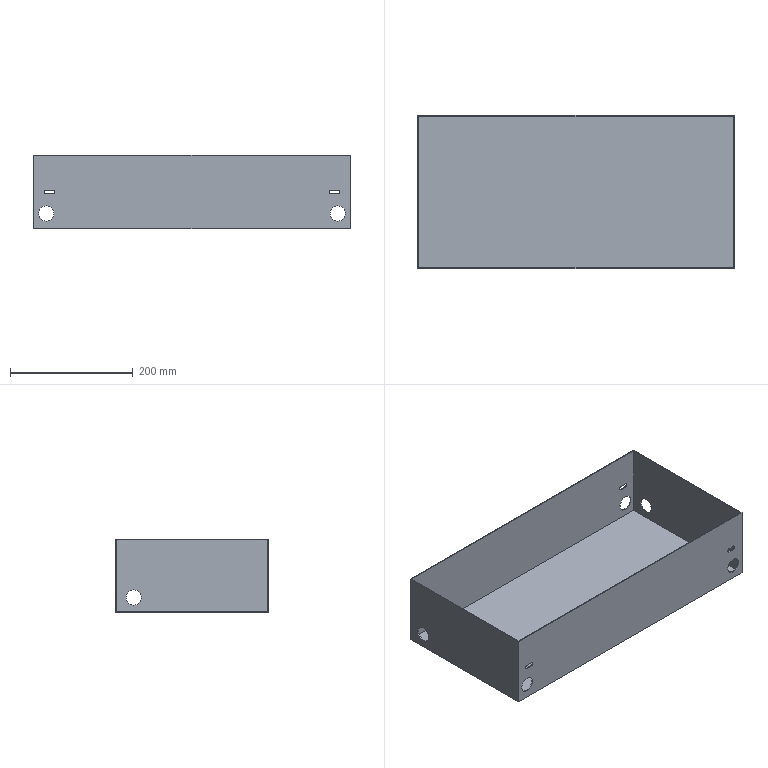Part | STEP file | ICT test machine electrical box | 1 solid | 39 faces | box 515 x 250 x 120 mm | volume 459009 mm3 | cylinder 20 | plane 19 | commonest cylinder face diameters 25 x12 6.5 x8